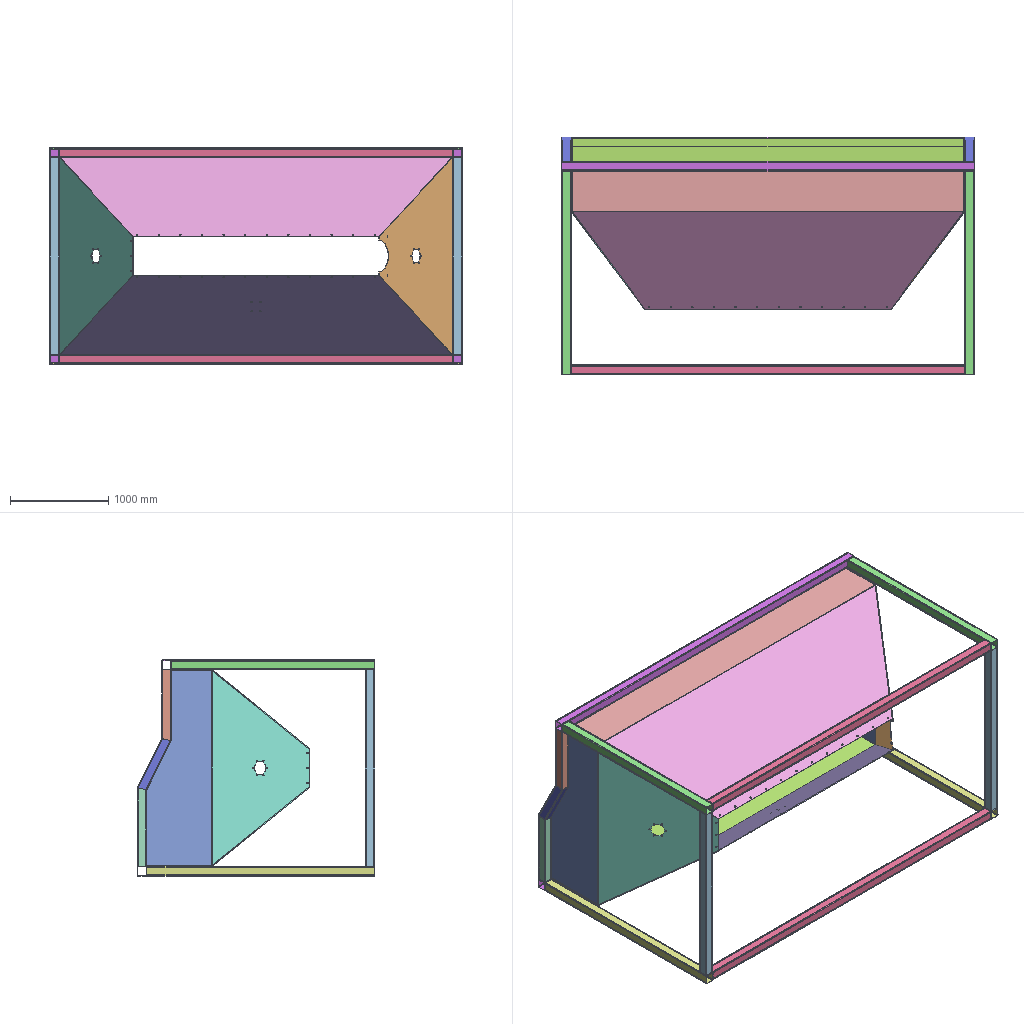Assembly | SolidWorks | 15 different items | 24 placed | box 4200 x 2420 x 2200 mm
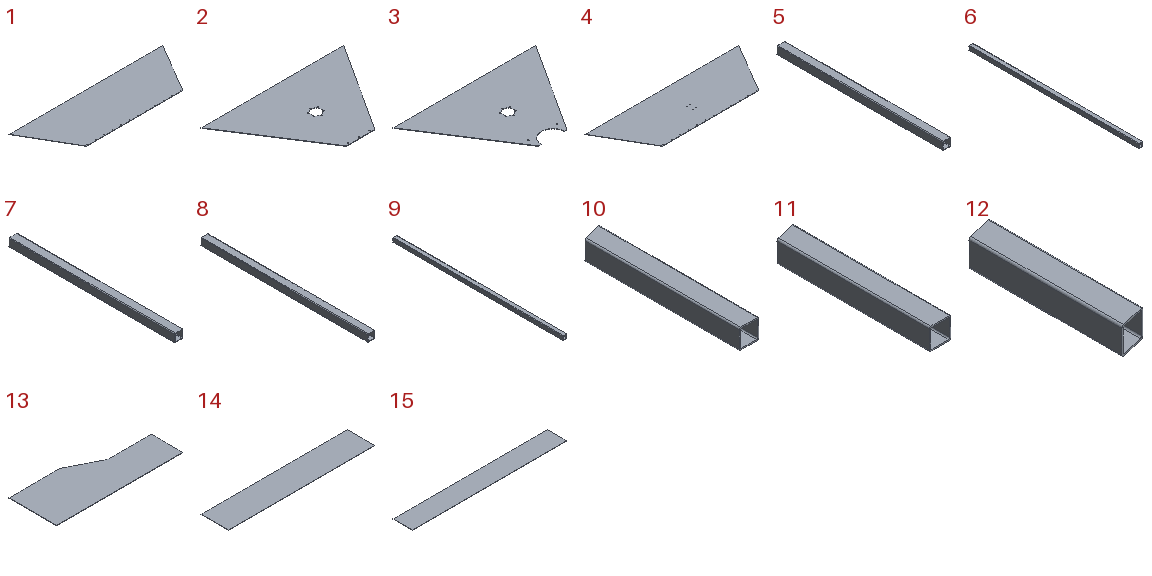Parts list (item | quantity | size | volume | features):
1 | x1 | 3983 x 1270 x 6 mm | 24689146 mm3 | features ICE 3, LPattern 2, FlatPattern 1, SMBaseFlange 1, SheetMetal 1
2 | x1 | 2000 x 1240 x 6 mm | 8830039 mm3 | features ICE 3, CirPattern 1, FlatPattern 1, SMBaseFlange 1, SheetMetal 1
3 | x1 | 2000 x 1240 x 6 mm | 8589688 mm3 | features ICE 4, CirPattern 1, FlatPattern 1, SMBaseFlange 1, SheetMetal 1
4 | x1 | 3983 x 1270 x 6 mm | 24685452 mm3 | features ICE 4, LPattern 2, FlatPattern 1, SMBaseFlange 1, SheetMetal 1
5 | x2 | 100 x 2070 x 100 mm | 4848096 mm3 | features Extrusion 1
6 | x2 | 100 x 4000 x 100 mm | 9368302 mm3 | features Extrusion 1
7 | x2 | 100 x 2000 x 100 mm | 4684151 mm3 | features Extrusion 1
8 | x2 | 100 x 2320 x 100 mm | 5433615 mm3 | features Extrusion 1
9 | x2 | 100 x 4200 x 100 mm | 9836717 mm3 | features Extrusion 1
10 | x2 | 100 x 800 x 100 mm | 1845556 mm3 | features Extrusion 1, ICE 1
11 | x2 | 100 x 723 x 100 mm | 1666387 mm3 | features Extrusion 1, ICE 1
12 | x2 | 100 x 582 x 100 mm | 1309220 mm3 | features Extrusion 1, ICE 1
13 | x2 | 1988 x 750 x 6 mm | 7533000 mm3 | features FlatPattern 1, ICE 1, SMBaseFlange 1, SheetMetal 1
14 | x1 | 4000 x 750 x 6 mm | 18000000 mm3 | features FlatPattern 1, SMBaseFlange 1, SheetMetal 1
15 | x1 | 4000 x 500 x 6 mm | 12000000 mm3 | features FlatPattern 1, SMBaseFlange 1, SheetMetal 1
Mates (type | each side: item.copy, entity, surface, feature):
Coincident | 5.1 face plane Boss-Extrude1 | 6.1 face plane Boss-Extrude1 | 3 times
Coincident | 5.2 face plane Boss-Extrude1 | 7.1 face plane Boss-Extrude1
Coincident | 7.1 face plane Boss-Extrude1 | 8.1 face plane Boss-Extrude1 | 3 times
Coincident | 6.1 face plane Boss-Extrude1 | 5.2 face plane Boss-Extrude1 | 3 times
Coincident | 6.2 face plane Boss-Extrude1 | 8.1 face plane Boss-Extrude1 | 3 times
Coincident | 7.1 face plane Boss-Extrude1 | 5.2 face plane Boss-Extrude1 | 2 times
Coincident | 6.2 face plane Boss-Extrude1 | 8.2 face plane Boss-Extrude1 | 3 times
Coincident | 5.1 face plane Boss-Extrude1 | 7.2 face plane Boss-Extrude1 | 3 times
Coincident | 6.1 face plane Boss-Extrude1 | assembly plane
Coincident | 7.1 plane | assembly plane
Coincident | 6.1 plane | assembly plane
Coincident | 5.2 face plane Boss-Extrude1 | 9.1 face plane Boss-Extrude1 | 3 times
Coincident | 8.1 face plane Boss-Extrude1 | 9.2 face plane Boss-Extrude1 | 3 times
Coincident | 9.2 face plane Boss-Extrude1 | 10.1 face plane Boss-Extrude1 | 2 times
Coincident | 8.1 face plane Boss-Extrude1 | 10.1 face plane Boss-Extrude1
Coincident | 9.1 face plane Boss-Extrude1 | 11.1 face plane Boss-Extrude1 | 2 times
Coincident | 5.2 face plane Boss-Extrude1 | 11.1 face plane Boss-Extrude1
Coincident | 11.1 face plane Boss-Extrude1 | 12.1 face plane Boss-Extrude1
Coincident | 10.1 edge | 12.1 edge
Coincident | 11.1 face plane Boss-Extrude1 | 12.1 edge
Coincident | 10.2 face plane Boss-Extrude1 | 12.2 face plane Boss-Extrude1
Coincident | 12.2 face plane Boss-Extrude1 | 11.2 face plane Boss-Extrude1
Coincident | 10.2 edge | 12.2 edge
Coincident | 9.1 face plane Boss-Extrude1 | 11.2 face plane Boss-Extrude1 | 2 times
Coincident | 9.2 face plane Boss-Extrude1 | 10.2 face plane Boss-Extrude1 | 2 times
Coincident | 12.2 edge | 11.2 face plane Boss-Extrude1
Coincident | 5.1 face plane Boss-Extrude1 | 11.2 face plane Boss-Extrude1
DistanceDim | 14.1 face plane Base-Flange1 | 9.2 face plane Boss-Extrude1
Coincident | 14.1 face plane Base-Flange1 | 9.2 face plane Boss-Extrude1
DistanceDim | 15.1 face plane Base-Flange1 | 9.1 face plane Boss-Extrude1
Coincident | 15.1 face plane Base-Flange1 | 9.1 face plane Boss-Extrude1
Coincident | 15.1 face plane Base-Flange1 | 11.2 face plane Boss-Extrude1
Coincident | 14.1 face plane Base-Flange1 | 10.2 face plane Boss-Extrude1
Coincident | 13.1 face plane Base-Flange1 | 10.1 face plane Boss-Extrude1
Coincident | 13.1 face plane Base-Flange1 | 14.1 face plane Base-Flange1 | 2 times
Coincident | 10.2 face plane Boss-Extrude1 | 13.2 face plane Base-Flange1
Coincident | 14.1 face plane Base-Flange1 | 13.2 face plane Base-Flange1 | 2 times
Coincident | 14.1 edge | 4.1 edge
Coincident | 15.1 edge | 1.1 edge
Coincident | 13.1 edge | 2.1 edge
DistanceDim | 1.1 edge | 4.1 edge
Coincident | 7.1 plane | 2.1 plane
Coincident | 6.1 plane | 1.1 plane
Coincident | 6.2 plane | 4.1 plane
Coincident | 1.1 vertex | 2.1 face plane Base-Flange1
Coincident | 4.1 vertex | 2.1 face plane Base-Flange1
DistanceDim | assembly face | 11.1 face plane Boss-Extrude1
Coincident | 2.1 plane | assembly plane | 2 times
Coincident | 2.1 face plane Base-Flange1 | assembly edge
Coincident | assembly face | assembly face | 7 times
DistanceDim | assembly face | assembly face | 3 times
Coincident | 7.2 face plane Boss-Extrude1 | assembly face | 3 times
DistanceDim | assembly axis | assembly axis | 2 times
DistanceDim | assembly axis | 8.2 face plane Boss-Extrude1
Coincident | 8.2 face plane Boss-Extrude1 | assembly face | 3 times
DistanceDim | assembly face | 11.2 face plane Boss-Extrude1
Symmetric | assembly face | assembly face | assembly plane
Symmetric | 5.1 face plane Boss-Extrude1 | 8.2 face plane Boss-Extrude1 | assembly plane
Coincident | 13.2 edge | 3.1 edge
Coincident | 2.1 plane | 3.1 plane
Coincident | 1.1 vertex | 3.1 face plane Base-Flange1
Coincident | 9.1 face plane Boss-Extrude1 | assembly face
Coincident | 9.1 edge | assembly plane | 2 times
Coincident | 9.2 face plane Boss-Extrude1 | assembly face
Coincident | 9.2 edge | assembly plane | 2 times
Parallel | 9.1 face plane Boss-Extrude1 | assembly face
Parallel | 9.2 face plane Boss-Extrude1 | assembly face
Coincident | 4.1 face plane Base-Flange1 | assembly face | 2 times
Coincident | 4.1 plane | assembly plane
Coincident | 2.1 face plane Base-Flange1 | assembly face
DistanceDim | assembly face | 4.1 edge
DistanceDim | assembly face | 2.1 edge
Concentric | 4.1 face cylinder Cut-Extrude4 | assembly face | 2 times
Coincident | 7.1 face plane Boss-Extrude1 | assembly face | 2 times
Tangent | 13.1 face plane Base-Flange1 | assembly face
Coincident | 13.1 select_type:24 | assembly plane
Perpendicular | 13.1 face plane Base-Flange1 | assembly plane
DistanceDim | 13.1 select_type:25 | assembly face
Tangent | 14.1 face plane Base-Flange1 | assembly face
Coincident | 14.1 select_type:24 | assembly face
Coincident | 14.1 select_type:24 | assembly plane
Tangent | 15.1 face plane Base-Flange1 | assembly face
Coincident | 15.1 select_type:24 | assembly plane | 2 times
Parallel | 15.1 face plane Base-Flange1 | assembly plane